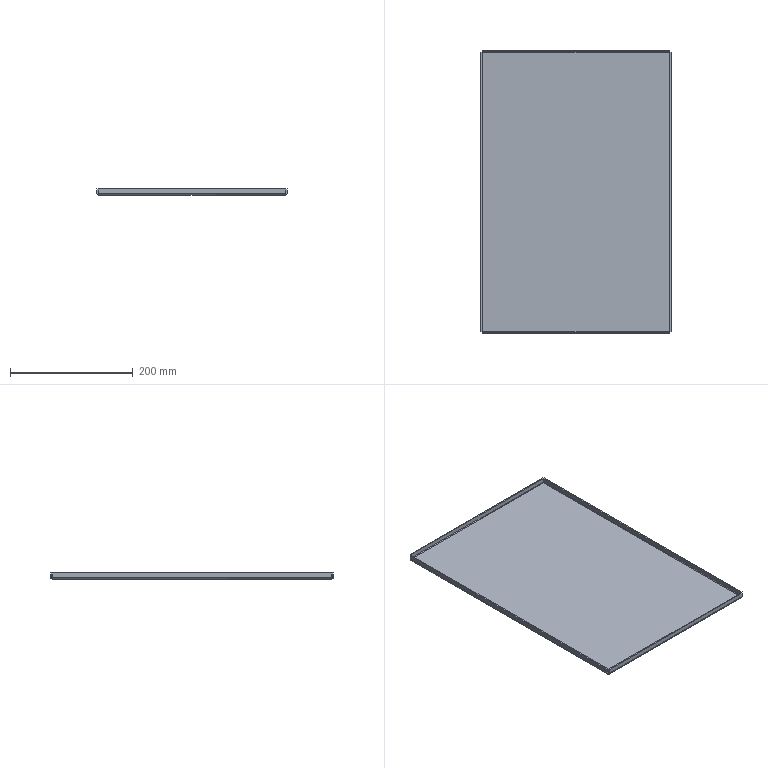Part | SolidWorks | features EdgeFlange 1, FlatPattern 1, SMBaseFlange 1, SheetMetal 1 | 1 solid | 38 faces | box 310 x 460 x 10 mm | volume 306822 mm3 | plane 22 | spline 8 | cylinder 8 | commonest cylinder face diameters 2 x4 6 x4
STEP:
#1=CARTESIAN_POINT('',(152.,-227.,-2.));
#2=VERTEX_POINT('',#1);
#3=CARTESIAN_POINT('',(-152.,-227.,-2.));
#4=VERTEX_POINT('',#3);
#5=CARTESIAN_POINT('',(152.293,-227.,-2.));
#6=DIRECTION('',(-1.,0.,0.));
#7=VECTOR('',#6,1000.);
#8=LINE('',#5,#7);
#9=EDGE_CURVE('',#2,#4,#8,.T.);
#10=ORIENTED_EDGE('',*,*,#9,.T.);
#11=CARTESIAN_POINT('',(-152.,227.,-2.));
#12=VERTEX_POINT('',#11);
#13=CARTESIAN_POINT('',(-152.,-227.293,-2.));
#14=DIRECTION('',(0.,1.,0.));
#15=VECTOR('',#14,1000.);
#16=LINE('',#13,#15);
#17=EDGE_CURVE('',#4,#12,#16,.T.);
#18=ORIENTED_EDGE('',*,*,#17,.T.);
#19=CARTESIAN_POINT('',(152.,227.,-2.));
#20=VERTEX_POINT('',#19);
#21=CARTESIAN_POINT('',(-152.293,227.,-2.));
#22=DIRECTION('',(1.,0.,0.));
#23=VECTOR('',#22,1000.);
#24=LINE('',#21,#23);
#25=EDGE_CURVE('',#12,#20,#24,.T.);
#26=ORIENTED_EDGE('',*,*,#25,.T.);
#27=CARTESIAN_POINT('',(152.,227.293,-2.));
#28=DIRECTION('',(0.,-1.,0.));
#29=VECTOR('',#28,1000.);
#30=LINE('',#27,#29);
#31=EDGE_CURVE('',#20,#2,#30,.T.);
#32=ORIENTED_EDGE('',*,*,#31,.T.);
#33=EDGE_LOOP('',(#10,#18,#26,#32));
#34=FACE_OUTER_BOUND('',#33,.T.);
#35=CARTESIAN_POINT('',(0.,0.,-2.));
#36=DIRECTION('',(0.,0.,1.));
#37=DIRECTION('',(1.,0.,0.));
#38=AXIS2_PLACEMENT_3D('',#35,#36,#37);
#39=PLANE('',#38);
#40=ADVANCED_FACE('',(#34),#39,.F.);
#41=CARTESIAN_POINT('',(-152.,-227.,0.));
#42=VERTEX_POINT('',#41);
#43=CARTESIAN_POINT('',(-152.,227.,0.));
#44=VERTEX_POINT('',#43);
#45=CARTESIAN_POINT('',(-152.,-227.293,0.));
#46=DIRECTION('',(0.,1.,0.));
#47=VECTOR('',#46,1000.);
#48=LINE('',#45,#47);
#49=EDGE_CURVE('',#42,#44,#48,.T.);
#50=ORIENTED_EDGE('',*,*,#49,.F.);
#51=CARTESIAN_POINT('',(152.,-227.,0.));
#52=VERTEX_POINT('',#51);
#53=CARTESIAN_POINT('',(152.293,-227.,0.));
#54=DIRECTION('',(-1.,0.,0.));
#55=VECTOR('',#54,1000.);
#56=LINE('',#53,#55);
#57=EDGE_CURVE('',#52,#42,#56,.T.);
#58=ORIENTED_EDGE('',*,*,#57,.F.);
#59=CARTESIAN_POINT('',(152.,227.,0.));
#60=VERTEX_POINT('',#59);
#61=CARTESIAN_POINT('',(152.,227.293,0.));
#62=DIRECTION('',(0.,-1.,0.));
#63=VECTOR('',#62,1000.);
#64=LINE('',#61,#63);
#65=EDGE_CURVE('',#60,#52,#64,.T.);
#66=ORIENTED_EDGE('',*,*,#65,.F.);
#67=CARTESIAN_POINT('',(-152.293,227.,0.));
#68=DIRECTION('',(1.,0.,0.));
#69=VECTOR('',#68,1000.);
#70=LINE('',#67,#69);
#71=EDGE_CURVE('',#44,#60,#70,.T.);
#72=ORIENTED_EDGE('',*,*,#71,.F.);
#73=EDGE_LOOP('',(#50,#58,#66,#72));
#74=FACE_OUTER_BOUND('',#73,.T.);
#75=CARTESIAN_POINT('',(0.,0.,0.));
#76=DIRECTION('',(0.,0.,1.));
#77=DIRECTION('',(1.,0.,0.));
#78=AXIS2_PLACEMENT_3D('',#75,#76,#77);
#79=PLANE('',#78);
#80=ADVANCED_FACE('',(#74),#79,.T.);
#81=CARTESIAN_POINT('',(-155.,227.293,1.));
#82=VERTEX_POINT('',#81);
#83=CARTESIAN_POINT('',(-153.,227.293,1.));
#84=VERTEX_POINT('',#83);
#85=CARTESIAN_POINT('',(-153.,227.293,1.));
#86=DIRECTION('',(1.,0.,0.));
#87=VECTOR('',#86,1000.);
#88=LINE('',#85,#87);
#89=EDGE_CURVE('',#82,#84,#88,.T.);
#90=ORIENTED_EDGE('',*,*,#89,.T.);
#91=CARTESIAN_POINT('',(-152.,227.,0.));
#92=CARTESIAN_POINT('',(-152.262,227.049,0.));
#93=CARTESIAN_POINT('',(-152.522,227.098,0.1078));
#94=CARTESIAN_POINT('',(-152.892,227.195,0.478));
#95=CARTESIAN_POINT('',(-153.,227.244,0.7382));
#96=CARTESIAN_POINT('',(-153.,227.293,1.));
#97=B_SPLINE_CURVE_WITH_KNOTS('',3,(#91,#92,#93,#94,#95,#96),.UNSPECIFIED.,.F.,.F.,(4,2,4),(0.,0.5,1.),.UNSPECIFIED.);
#98=EDGE_CURVE('',#44,#84,#97,.T.);
#99=ORIENTED_EDGE('',*,*,#98,.F.);
#100=CARTESIAN_POINT('',(-152.,227.,0.));
#101=DIRECTION('',(0.,0.,-1.));
#102=VECTOR('',#101,1000.);
#103=LINE('',#100,#102);
#104=EDGE_CURVE('',#44,#12,#103,.T.);
#105=ORIENTED_EDGE('',*,*,#104,.T.);
#106=CARTESIAN_POINT('',(-152.,227.,-2.));
#107=CARTESIAN_POINT('',(-152.393,227.024,-2.));
#108=CARTESIAN_POINT('',(-152.785,227.049,-1.922));
#109=CARTESIAN_POINT('',(-153.511,227.098,-1.621));
#110=CARTESIAN_POINT('',(-153.844,227.122,-1.399));
#111=CARTESIAN_POINT('',(-154.399,227.171,-0.8436));
#112=CARTESIAN_POINT('',(-154.621,227.195,-0.5109));
#113=CARTESIAN_POINT('',(-154.922,227.244,0.2148));
#114=CARTESIAN_POINT('',(-155.,227.268,0.6073));
#115=CARTESIAN_POINT('',(-155.,227.293,1.));
#116=B_SPLINE_CURVE_WITH_KNOTS('',3,(#106,#107,#108,#109,#110,#111,#112,#113,#114,#115),.UNSPECIFIED.,.F.,.F.,(4,2,2,2,4),(0.,0.25,0.5,0.75,1.),.UNSPECIFIED.);
#117=EDGE_CURVE('',#12,#82,#116,.T.);
#118=ORIENTED_EDGE('',*,*,#117,.T.);
#119=EDGE_LOOP('',(#90,#99,#105,#118));
#120=FACE_OUTER_BOUND('',#119,.T.);
#121=CARTESIAN_POINT('',(-152.,227.,-2.02));
#122=CARTESIAN_POINT('',(-152.395,227.024,-2.02));
#123=CARTESIAN_POINT('',(-152.79,227.049,-1.941));
#124=CARTESIAN_POINT('',(-153.521,227.098,-1.639));
#125=CARTESIAN_POINT('',(-153.856,227.122,-1.415));
#126=CARTESIAN_POINT('',(-154.415,227.171,-0.8559));
#127=CARTESIAN_POINT('',(-154.639,227.195,-0.5209));
#128=CARTESIAN_POINT('',(-154.941,227.244,0.2095));
#129=CARTESIAN_POINT('',(-155.02,227.268,0.6046));
#130=CARTESIAN_POINT('',(-155.02,227.293,1.));
#131=CARTESIAN_POINT('',(-152.,227.,-2.));
#132=CARTESIAN_POINT('',(-152.393,227.024,-2.));
#133=CARTESIAN_POINT('',(-152.785,227.049,-1.922));
#134=CARTESIAN_POINT('',(-153.511,227.098,-1.621));
#135=CARTESIAN_POINT('',(-153.844,227.122,-1.399));
#136=CARTESIAN_POINT('',(-154.399,227.171,-0.8436));
#137=CARTESIAN_POINT('',(-154.621,227.195,-0.5109));
#138=CARTESIAN_POINT('',(-154.922,227.244,0.2148));
#139=CARTESIAN_POINT('',(-155.,227.268,0.6072));
#140=CARTESIAN_POINT('',(-155.,227.293,1.));
#141=CARTESIAN_POINT('',(-152.,227.,0.));
#142=CARTESIAN_POINT('',(-152.131,227.024,0.));
#143=CARTESIAN_POINT('',(-152.262,227.049,0.02603));
#144=CARTESIAN_POINT('',(-152.504,227.098,0.1262));
#145=CARTESIAN_POINT('',(-152.615,227.122,0.2003));
#146=CARTESIAN_POINT('',(-152.8,227.171,0.3855));
#147=CARTESIAN_POINT('',(-152.874,227.195,0.4964));
#148=CARTESIAN_POINT('',(-152.974,227.244,0.7383));
#149=CARTESIAN_POINT('',(-153.,227.268,0.8691));
#150=CARTESIAN_POINT('',(-153.,227.293,1.));
#151=CARTESIAN_POINT('',(-152.,227.,0.0202));
#152=CARTESIAN_POINT('',(-152.128,227.024,0.0202));
#153=CARTESIAN_POINT('',(-152.256,227.049,0.0457));
#154=CARTESIAN_POINT('',(-152.493,227.098,0.1439));
#155=CARTESIAN_POINT('',(-152.602,227.122,0.2165));
#156=CARTESIAN_POINT('',(-152.784,227.171,0.3979));
#157=CARTESIAN_POINT('',(-152.856,227.195,0.5066));
#158=CARTESIAN_POINT('',(-152.954,227.244,0.7435));
#159=CARTESIAN_POINT('',(-152.98,227.268,0.8717));
#160=CARTESIAN_POINT('',(-152.98,227.293,1.));
#161=B_SPLINE_SURFACE_WITH_KNOTS('',1,3,((#121,#122,#123,#124,#125,#126,#127,#128,#129,#130),(#131,#132,#133,#134,#135,#136,#137,#138,#139,#140),(#141,#142,#143,#144,#145,#146,#147,#148,#149,#150),(#151,#152,#153,#154,#155,#156,#157,#158,#159,#160)),.UNSPECIFIED.,.F.,.F.,.F.,(2,1,1,2),(4,2,2,2,4),(-0.01,0.,1.,1.01),(0.,0.25,0.5,0.75,1.),.UNSPECIFIED.);
#162=ADVANCED_FACE('',(#120),#161,.F.);
#163=CARTESIAN_POINT('',(-153.,-227.293,1.));
#164=VERTEX_POINT('',#163);
#165=CARTESIAN_POINT('',(-153.,-227.293,1.));
#166=CARTESIAN_POINT('',(-153.,-227.244,0.7382));
#167=CARTESIAN_POINT('',(-152.892,-227.195,0.478));
#168=CARTESIAN_POINT('',(-152.522,-227.098,0.1078));
#169=CARTESIAN_POINT('',(-152.262,-227.049,0.));
#170=CARTESIAN_POINT('',(-152.,-227.,0.));
#171=B_SPLINE_CURVE_WITH_KNOTS('',3,(#165,#166,#167,#168,#169,#170),.UNSPECIFIED.,.F.,.F.,(4,2,4),(0.,0.5,1.),.UNSPECIFIED.);
#172=EDGE_CURVE('',#164,#42,#171,.T.);
#173=ORIENTED_EDGE('',*,*,#172,.F.);
#174=CARTESIAN_POINT('',(-155.,-227.293,1.));
#175=VERTEX_POINT('',#174);
#176=CARTESIAN_POINT('',(-153.,-227.293,1.));
#177=DIRECTION('',(1.,0.,0.));
#178=VECTOR('',#177,1000.);
#179=LINE('',#176,#178);
#180=EDGE_CURVE('',#175,#164,#179,.T.);
#181=ORIENTED_EDGE('',*,*,#180,.F.);
#182=CARTESIAN_POINT('',(-155.,-227.293,1.));
#183=CARTESIAN_POINT('',(-155.,-227.268,0.6073));
#184=CARTESIAN_POINT('',(-154.922,-227.244,0.2148));
#185=CARTESIAN_POINT('',(-154.621,-227.195,-0.5109));
#186=CARTESIAN_POINT('',(-154.399,-227.171,-0.8436));
#187=CARTESIAN_POINT('',(-153.844,-227.122,-1.399));
#188=CARTESIAN_POINT('',(-153.511,-227.098,-1.621));
#189=CARTESIAN_POINT('',(-152.785,-227.049,-1.922));
#190=CARTESIAN_POINT('',(-152.393,-227.024,-2.));
#191=CARTESIAN_POINT('',(-152.,-227.,-2.));
#192=B_SPLINE_CURVE_WITH_KNOTS('',3,(#182,#183,#184,#185,#186,#187,#188,#189,#190,#191),.UNSPECIFIED.,.F.,.F.,(4,2,2,2,4),(0.,0.25,0.5,0.75,1.),.UNSPECIFIED.);
#193=EDGE_CURVE('',#175,#4,#192,.T.);
#194=ORIENTED_EDGE('',*,*,#193,.T.);
#195=CARTESIAN_POINT('',(-152.,-227.,0.));
#196=DIRECTION('',(0.,0.,-1.));
#197=VECTOR('',#196,1000.);
#198=LINE('',#195,#197);
#199=EDGE_CURVE('',#42,#4,#198,.T.);
#200=ORIENTED_EDGE('',*,*,#199,.F.);
#201=EDGE_LOOP('',(#173,#181,#194,#200));
#202=FACE_OUTER_BOUND('',#201,.T.);
#203=CARTESIAN_POINT('',(-155.02,-227.293,1.));
#204=CARTESIAN_POINT('',(-155.02,-227.268,0.6046));
#205=CARTESIAN_POINT('',(-154.941,-227.244,0.2095));
#206=CARTESIAN_POINT('',(-154.639,-227.195,-0.5209));
#207=CARTESIAN_POINT('',(-154.415,-227.171,-0.8559));
#208=CARTESIAN_POINT('',(-153.856,-227.122,-1.415));
#209=CARTESIAN_POINT('',(-153.521,-227.098,-1.639));
#210=CARTESIAN_POINT('',(-152.79,-227.049,-1.941));
#211=CARTESIAN_POINT('',(-152.395,-227.024,-2.02));
#212=CARTESIAN_POINT('',(-152.,-227.,-2.02));
#213=CARTESIAN_POINT('',(-155.,-227.293,1.));
#214=CARTESIAN_POINT('',(-155.,-227.268,0.6072));
#215=CARTESIAN_POINT('',(-154.922,-227.244,0.2148));
#216=CARTESIAN_POINT('',(-154.621,-227.195,-0.5109));
#217=CARTESIAN_POINT('',(-154.399,-227.171,-0.8436));
#218=CARTESIAN_POINT('',(-153.844,-227.122,-1.399));
#219=CARTESIAN_POINT('',(-153.511,-227.098,-1.621));
#220=CARTESIAN_POINT('',(-152.785,-227.049,-1.922));
#221=CARTESIAN_POINT('',(-152.393,-227.024,-2.));
#222=CARTESIAN_POINT('',(-152.,-227.,-2.));
#223=CARTESIAN_POINT('',(-153.,-227.293,1.));
#224=CARTESIAN_POINT('',(-153.,-227.268,0.8691));
#225=CARTESIAN_POINT('',(-152.974,-227.244,0.7383));
#226=CARTESIAN_POINT('',(-152.874,-227.195,0.4964));
#227=CARTESIAN_POINT('',(-152.8,-227.171,0.3855));
#228=CARTESIAN_POINT('',(-152.615,-227.122,0.2003));
#229=CARTESIAN_POINT('',(-152.504,-227.098,0.1262));
#230=CARTESIAN_POINT('',(-152.262,-227.049,0.02603));
#231=CARTESIAN_POINT('',(-152.131,-227.024,0.));
#232=CARTESIAN_POINT('',(-152.,-227.,0.));
#233=CARTESIAN_POINT('',(-152.98,-227.293,1.));
#234=CARTESIAN_POINT('',(-152.98,-227.268,0.8717));
#235=CARTESIAN_POINT('',(-152.954,-227.244,0.7435));
#236=CARTESIAN_POINT('',(-152.856,-227.195,0.5066));
#237=CARTESIAN_POINT('',(-152.784,-227.171,0.3979));
#238=CARTESIAN_POINT('',(-152.602,-227.122,0.2165));
#239=CARTESIAN_POINT('',(-152.493,-227.098,0.1439));
#240=CARTESIAN_POINT('',(-152.256,-227.049,0.0457));
#241=CARTESIAN_POINT('',(-152.128,-227.024,0.0202));
#242=CARTESIAN_POINT('',(-152.,-227.,0.0202));
#243=B_SPLINE_SURFACE_WITH_KNOTS('',1,3,((#203,#204,#205,#206,#207,#208,#209,#210,#211,#212),(#213,#214,#215,#216,#217,#218,#219,#220,#221,#222),(#223,#224,#225,#226,#227,#228,#229,#230,#231,#232),(#233,#234,#235,#236,#237,#238,#239,#240,#241,#242)),.UNSPECIFIED.,.F.,.F.,.F.,(2,1,1,2),(4,2,2,2,4),(-0.01,0.,1.,1.01),(0.,0.25,0.5,0.75,1.),.UNSPECIFIED.);
#244=ADVANCED_FACE('',(#202),#243,.F.);
#245=ORIENTED_EDGE('',*,*,#17,.F.);
#246=ORIENTED_EDGE('',*,*,#193,.F.);
#247=CARTESIAN_POINT('',(-155.,230.,1.));
#248=DIRECTION('',(0.,1.,0.));
#249=VECTOR('',#248,1000.);
#250=LINE('',#247,#249);
#251=EDGE_CURVE('',#175,#82,#250,.T.);
#252=ORIENTED_EDGE('',*,*,#251,.T.);
#253=ORIENTED_EDGE('',*,*,#117,.F.);
#254=EDGE_LOOP('',(#245,#246,#252,#253));
#255=FACE_OUTER_BOUND('',#254,.T.);
#256=CARTESIAN_POINT('',(-152.,-227.293,1.));
#257=DIRECTION('',(0.,-1.,0.));
#258=DIRECTION('',(-1.,0.,0.));
#259=AXIS2_PLACEMENT_3D('',#256,#257,#258);
#260=CYLINDRICAL_SURFACE('',#259,3.);
#261=ADVANCED_FACE('',(#255),#260,.T.);
#262=ORIENTED_EDGE('',*,*,#49,.T.);
#263=ORIENTED_EDGE('',*,*,#98,.T.);
#264=CARTESIAN_POINT('',(-153.,230.,1.));
#265=DIRECTION('',(0.,-1.,0.));
#266=VECTOR('',#265,1000.);
#267=LINE('',#264,#266);
#268=EDGE_CURVE('',#84,#164,#267,.T.);
#269=ORIENTED_EDGE('',*,*,#268,.T.);
#270=ORIENTED_EDGE('',*,*,#172,.T.);
#271=EDGE_LOOP('',(#262,#263,#269,#270));
#272=FACE_OUTER_BOUND('',#271,.T.);
#273=CARTESIAN_POINT('',(-152.,-227.293,1.));
#274=DIRECTION('',(0.,-1.,0.));
#275=DIRECTION('',(-1.,0.,0.));
#276=AXIS2_PLACEMENT_3D('',#273,#274,#275);
#277=CYLINDRICAL_SURFACE('',#276,1.);
#278=ADVANCED_FACE('',(#272),#277,.F.);
#279=CARTESIAN_POINT('',(-155.,227.293,8.));
#280=VERTEX_POINT('',#279);
#281=CARTESIAN_POINT('',(-155.,227.293,0.));
#282=DIRECTION('',(0.,0.,1.));
#283=VECTOR('',#282,1000.);
#284=LINE('',#281,#283);
#285=EDGE_CURVE('',#82,#280,#284,.T.);
#286=ORIENTED_EDGE('',*,*,#285,.T.);
#287=CARTESIAN_POINT('',(-153.,227.293,8.));
#288=VERTEX_POINT('',#287);
#289=CARTESIAN_POINT('',(-153.,227.293,8.));
#290=DIRECTION('',(1.,0.,0.));
#291=VECTOR('',#290,1000.);
#292=LINE('',#289,#291);
#293=EDGE_CURVE('',#280,#288,#292,.T.);
#294=ORIENTED_EDGE('',*,*,#293,.T.);
#295=CARTESIAN_POINT('',(-153.,227.293,0.));
#296=DIRECTION('',(0.,0.,1.));
#297=VECTOR('',#296,1000.);
#298=LINE('',#295,#297);
#299=EDGE_CURVE('',#84,#288,#298,.T.);
#300=ORIENTED_EDGE('',*,*,#299,.F.);
#301=ORIENTED_EDGE('',*,*,#89,.F.);
#302=EDGE_LOOP('',(#286,#294,#300,#301));
#303=FACE_OUTER_BOUND('',#302,.T.);
#304=CARTESIAN_POINT('',(-153.,227.293,0.));
#305=DIRECTION('',(0.,1.,0.));
#306=DIRECTION('',(0.,0.,1.));
#307=AXIS2_PLACEMENT_3D('',#304,#305,#306);
#308=PLANE('',#307);
#309=ADVANCED_FACE('',(#303),#308,.T.);
#310=ORIENTED_EDGE('',*,*,#251,.F.);
#311=CARTESIAN_POINT('',(-155.,-227.293,8.));
#312=VERTEX_POINT('',#311);
#313=CARTESIAN_POINT('',(-155.,-227.293,0.));
#314=DIRECTION('',(0.,0.,1.));
#315=VECTOR('',#314,1000.);
#316=LINE('',#313,#315);
#317=EDGE_CURVE('',#175,#312,#316,.T.);
#318=ORIENTED_EDGE('',*,*,#317,.T.);
#319=CARTESIAN_POINT('',(-155.,0.,8.));
#320=DIRECTION('',(0.,1.,0.));
#321=VECTOR('',#320,1000.);
#322=LINE('',#319,#321);
#323=EDGE_CURVE('',#312,#280,#322,.T.);
#324=ORIENTED_EDGE('',*,*,#323,.T.);
#325=ORIENTED_EDGE('',*,*,#285,.F.);
#326=EDGE_LOOP('',(#310,#318,#324,#325));
#327=FACE_OUTER_BOUND('',#326,.T.);
#328=CARTESIAN_POINT('',(-155.,0.,0.));
#329=DIRECTION('',(1.,0.,0.));
#330=DIRECTION('',(0.,0.,-1.));
#331=AXIS2_PLACEMENT_3D('',#328,#329,#330);
#332=PLANE('',#331);
#333=ADVANCED_FACE('',(#327),#332,.F.);
#334=CARTESIAN_POINT('',(-153.,-227.293,8.));
#335=VERTEX_POINT('',#334);
#336=CARTESIAN_POINT('',(-153.,-227.293,0.));
#337=DIRECTION('',(0.,0.,1.));
#338=VECTOR('',#337,1000.);
#339=LINE('',#336,#338);
#340=EDGE_CURVE('',#164,#335,#339,.T.);
#341=ORIENTED_EDGE('',*,*,#340,.F.);
#342=ORIENTED_EDGE('',*,*,#268,.F.);
#343=ORIENTED_EDGE('',*,*,#299,.T.);
#344=CARTESIAN_POINT('',(-153.,230.,8.));
#345=DIRECTION('',(0.,1.,0.));
#346=VECTOR('',#345,1000.);
#347=LINE('',#344,#346);
#348=EDGE_CURVE('',#335,#288,#347,.T.);
#349=ORIENTED_EDGE('',*,*,#348,.F.);
#350=EDGE_LOOP('',(#341,#342,#343,#349));
#351=FACE_OUTER_BOUND('',#350,.T.);
#352=CARTESIAN_POINT('',(-153.,0.,0.));
#353=DIRECTION('',(1.,0.,0.));
#354=DIRECTION('',(0.,0.,-1.));
#355=AXIS2_PLACEMENT_3D('',#352,#353,#354);
#356=PLANE('',#355);
#357=ADVANCED_FACE('',(#351),#356,.T.);
#358=ORIENTED_EDGE('',*,*,#323,.F.);
#359=CARTESIAN_POINT('',(-155.,-227.293,8.));
#360=DIRECTION('',(1.,0.,0.));
#361=VECTOR('',#360,1000.);
#362=LINE('',#359,#361);
#363=EDGE_CURVE('',#312,#335,#362,.T.);
#364=ORIENTED_EDGE('',*,*,#363,.T.);
#365=ORIENTED_EDGE('',*,*,#348,.T.);
#366=ORIENTED_EDGE('',*,*,#293,.F.);
#367=EDGE_LOOP('',(#358,#364,#365,#366));
#368=FACE_OUTER_BOUND('',#367,.T.);
#369=CARTESIAN_POINT('',(-155.,230.,8.));
#370=DIRECTION('',(0.,0.,-1.));
#371=DIRECTION('',(-1.,0.,0.));
#372=AXIS2_PLACEMENT_3D('',#369,#370,#371);
#373=PLANE('',#372);
#374=ADVANCED_FACE('',(#368),#373,.F.);
#375=ORIENTED_EDGE('',*,*,#363,.F.);
#376=ORIENTED_EDGE('',*,*,#317,.F.);
#377=ORIENTED_EDGE('',*,*,#180,.T.);
#378=ORIENTED_EDGE('',*,*,#340,.T.);
#379=EDGE_LOOP('',(#375,#376,#377,#378));
#380=FACE_OUTER_BOUND('',#379,.T.);
#381=CARTESIAN_POINT('',(-153.,-227.293,0.));
#382=DIRECTION('',(0.,1.,0.));
#383=DIRECTION('',(0.,0.,1.));
#384=AXIS2_PLACEMENT_3D('',#381,#382,#383);
#385=PLANE('',#384);
#386=ADVANCED_FACE('',(#380),#385,.F.);
#387=CARTESIAN_POINT('',(152.293,230.,1.));
#388=VERTEX_POINT('',#387);
#389=CARTESIAN_POINT('',(152.293,228.,1.));
#390=VERTEX_POINT('',#389);
#391=CARTESIAN_POINT('',(152.293,228.,1.));
#392=DIRECTION('',(0.,-1.,0.));
#393=VECTOR('',#392,1000.);
#394=LINE('',#391,#393);
#395=EDGE_CURVE('',#388,#390,#394,.T.);
#396=ORIENTED_EDGE('',*,*,#395,.T.);
#397=CARTESIAN_POINT('',(152.,227.,0.));
#398=CARTESIAN_POINT('',(152.049,227.262,0.));
#399=CARTESIAN_POINT('',(152.098,227.522,0.1078));
#400=CARTESIAN_POINT('',(152.195,227.892,0.478));
#401=CARTESIAN_POINT('',(152.244,228.,0.7382));
#402=CARTESIAN_POINT('',(152.293,228.,1.));
#403=B_SPLINE_CURVE_WITH_KNOTS('',3,(#397,#398,#399,#400,#401,#402),.UNSPECIFIED.,.F.,.F.,(4,2,4),(0.,0.5,1.),.UNSPECIFIED.);
#404=EDGE_CURVE('',#60,#390,#403,.T.);
#405=ORIENTED_EDGE('',*,*,#404,.F.);
#406=CARTESIAN_POINT('',(152.,227.,0.));
#407=DIRECTION('',(0.,0.,-1.));
#408=VECTOR('',#407,1000.);
#409=LINE('',#406,#408);
#410=EDGE_CURVE('',#60,#20,#409,.T.);
#411=ORIENTED_EDGE('',*,*,#410,.T.);
#412=CARTESIAN_POINT('',(152.,227.,-2.));
#413=CARTESIAN_POINT('',(152.024,227.393,-2.));
#414=CARTESIAN_POINT('',(152.049,227.785,-1.922));
#415=CARTESIAN_POINT('',(152.098,228.511,-1.621));
#416=CARTESIAN_POINT('',(152.122,228.844,-1.399));
#417=CARTESIAN_POINT('',(152.171,229.399,-0.8436));
#418=CARTESIAN_POINT('',(152.195,229.621,-0.5109));
#419=CARTESIAN_POINT('',(152.244,229.922,0.2148));
#420=CARTESIAN_POINT('',(152.268,230.,0.6073));
#421=CARTESIAN_POINT('',(152.293,230.,1.));
#422=B_SPLINE_CURVE_WITH_KNOTS('',3,(#412,#413,#414,#415,#416,#417,#418,#419,#420,#421),.UNSPECIFIED.,.F.,.F.,(4,2,2,2,4),(0.,0.25,0.5,0.75,1.),.UNSPECIFIED.);
#423=EDGE_CURVE('',#20,#388,#422,.T.);
#424=ORIENTED_EDGE('',*,*,#423,.T.);
#425=EDGE_LOOP('',(#396,#405,#411,#424));
#426=FACE_OUTER_BOUND('',#425,.T.);
#427=CARTESIAN_POINT('',(152.,227.,-2.02));
#428=CARTESIAN_POINT('',(152.024,227.395,-2.02));
#429=CARTESIAN_POINT('',(152.049,227.79,-1.941));
#430=CARTESIAN_POINT('',(152.098,228.521,-1.639));
#431=CARTESIAN_POINT('',(152.122,228.856,-1.415));
#432=CARTESIAN_POINT('',(152.171,229.415,-0.8559));
#433=CARTESIAN_POINT('',(152.195,229.639,-0.5209));
#434=CARTESIAN_POINT('',(152.244,229.941,0.2095));
#435=CARTESIAN_POINT('',(152.268,230.02,0.6046));
#436=CARTESIAN_POINT('',(152.293,230.02,1.));
#437=CARTESIAN_POINT('',(152.,227.,-2.));
#438=CARTESIAN_POINT('',(152.024,227.393,-2.));
#439=CARTESIAN_POINT('',(152.049,227.785,-1.922));
#440=CARTESIAN_POINT('',(152.098,228.511,-1.621));
#441=CARTESIAN_POINT('',(152.122,228.844,-1.399));
#442=CARTESIAN_POINT('',(152.171,229.399,-0.8436));
#443=CARTESIAN_POINT('',(152.195,229.621,-0.5109));
#444=CARTESIAN_POINT('',(152.244,229.922,0.2148));
#445=CARTESIAN_POINT('',(152.268,230.,0.6072));
#446=CARTESIAN_POINT('',(152.293,230.,1.));
#447=CARTESIAN_POINT('',(152.,227.,0.));
#448=CARTESIAN_POINT('',(152.024,227.131,0.));
#449=CARTESIAN_POINT('',(152.049,227.262,0.02603));
#450=CARTESIAN_POINT('',(152.098,227.504,0.1262));
#451=CARTESIAN_POINT('',(152.122,227.615,0.2003));
#452=CARTESIAN_POINT('',(152.171,227.8,0.3855));
#453=CARTESIAN_POINT('',(152.195,227.874,0.4964));
#454=CARTESIAN_POINT('',(152.244,227.974,0.7383));
#455=CARTESIAN_POINT('',(152.268,228.,0.8691));
#456=CARTESIAN_POINT('',(152.293,228.,1.));
#457=CARTESIAN_POINT('',(152.,227.,0.0202));
#458=CARTESIAN_POINT('',(152.024,227.128,0.0202));
#459=CARTESIAN_POINT('',(152.049,227.256,0.0457));
#460=CARTESIAN_POINT('',(152.098,227.493,0.1439));
#461=CARTESIAN_POINT('',(152.122,227.602,0.2165));
#462=CARTESIAN_POINT('',(152.171,227.784,0.3979));
#463=CARTESIAN_POINT('',(152.195,227.856,0.5066));
#464=CARTESIAN_POINT('',(152.244,227.954,0.7435));
#465=CARTESIAN_POINT('',(152.268,227.98,0.8717));
#466=CARTESIAN_POINT('',(152.293,227.98,1.));
#467=B_SPLINE_SURFACE_WITH_KNOTS('',1,3,((#427,#428,#429,#430,#431,#432,#433,#434,#435,#436),(#437,#438,#439,#440,#441,#442,#443,#444,#445,#446),(#447,#448,#449,#450,#451,#452,#453,#454,#455,#456),(#457,#458,#459,#460,#461,#462,#463,#464,#465,#466)),.UNSPECIFIED.,.F.,.F.,.F.,(2,1,1,2),(4,2,2,2,4),(-0.01,0.,1.,1.01),(0.,0.25,0.5,0.75,1.),.UNSPECIFIED.);
#468=ADVANCED_FACE('',(#426),#467,.F.);
#469=CARTESIAN_POINT('',(-152.293,228.,1.));
#470=VERTEX_POINT('',#469);
#471=CARTESIAN_POINT('',(-152.293,228.,1.));
#472=CARTESIAN_POINT('',(-152.244,228.,0.7382));
#473=CARTESIAN_POINT('',(-152.195,227.892,0.478));
#474=CARTESIAN_POINT('',(-152.098,227.522,0.1078));
#475=CARTESIAN_POINT('',(-152.049,227.262,0.));
#476=CARTESIAN_POINT('',(-152.,227.,0.));
#477=B_SPLINE_CURVE_WITH_KNOTS('',3,(#471,#472,#473,#474,#475,#476),.UNSPECIFIED.,.F.,.F.,(4,2,4),(0.,0.5,1.),.UNSPECIFIED.);
#478=EDGE_CURVE('',#470,#44,#477,.T.);
#479=ORIENTED_EDGE('',*,*,#478,.F.);
#480=CARTESIAN_POINT('',(-152.293,230.,1.));
#481=VERTEX_POINT('',#480);
#482=CARTESIAN_POINT('',(-152.293,228.,1.));
#483=DIRECTION('',(0.,-1.,0.));
#484=VECTOR('',#483,1000.);
#485=LINE('',#482,#484);
#486=EDGE_CURVE('',#481,#470,#485,.T.);
#487=ORIENTED_EDGE('',*,*,#486,.F.);
#488=CARTESIAN_POINT('',(-152.293,230.,1.));
#489=CARTESIAN_POINT('',(-152.268,230.,0.6073));
#490=CARTESIAN_POINT('',(-152.244,229.922,0.2148));
#491=CARTESIAN_POINT('',(-152.195,229.621,-0.5109));
#492=CARTESIAN_POINT('',(-152.171,229.399,-0.8436));
#493=CARTESIAN_POINT('',(-152.122,228.844,-1.399));
#494=CARTESIAN_POINT('',(-152.098,228.511,-1.621));
#495=CARTESIAN_POINT('',(-152.049,227.785,-1.922));
#496=CARTESIAN_POINT('',(-152.024,227.393,-2.));
#497=CARTESIAN_POINT('',(-152.,227.,-2.));
#498=B_SPLINE_CURVE_WITH_KNOTS('',3,(#488,#489,#490,#491,#492,#493,#494,#495,#496,#497),.UNSPECIFIED.,.F.,.F.,(4,2,2,2,4),(0.,0.25,0.5,0.75,1.),.UNSPECIFIED.);
#499=EDGE_CURVE('',#481,#12,#498,.T.);
#500=ORIENTED_EDGE('',*,*,#499,.T.);
#501=ORIENTED_EDGE('',*,*,#104,.F.);
#502=EDGE_LOOP('',(#479,#487,#500,#501));
#503=FACE_OUTER_BOUND('',#502,.T.);
#504=CARTESIAN_POINT('',(-152.293,230.02,1.));
#505=CARTESIAN_POINT('',(-152.268,230.02,0.6046));
#506=CARTESIAN_POINT('',(-152.244,229.941,0.2095));
#507=CARTESIAN_POINT('',(-152.195,229.639,-0.5209));
#508=CARTESIAN_POINT('',(-152.171,229.415,-0.8559));
#509=CARTESIAN_POINT('',(-152.122,228.856,-1.415));
#510=CARTESIAN_POINT('',(-152.098,228.521,-1.639));
#511=CARTESIAN_POINT('',(-152.049,227.79,-1.941));
#512=CARTESIAN_POINT('',(-152.024,227.395,-2.02));
#513=CARTESIAN_POINT('',(-152.,227.,-2.02));
#514=CARTESIAN_POINT('',(-152.293,230.,1.));
#515=CARTESIAN_POINT('',(-152.268,230.,0.6072));
#516=CARTESIAN_POINT('',(-152.244,229.922,0.2148));
#517=CARTESIAN_POINT('',(-152.195,229.621,-0.5109));
#518=CARTESIAN_POINT('',(-152.171,229.399,-0.8436));
#519=CARTESIAN_POINT('',(-152.122,228.844,-1.399));
#520=CARTESIAN_POINT('',(-152.098,228.511,-1.621));
#521=CARTESIAN_POINT('',(-152.049,227.785,-1.922));
#522=CARTESIAN_POINT('',(-152.024,227.393,-2.));
#523=CARTESIAN_POINT('',(-152.,227.,-2.));
#524=CARTESIAN_POINT('',(-152.293,228.,1.));
#525=CARTESIAN_POINT('',(-152.268,228.,0.8691));
#526=CARTESIAN_POINT('',(-152.244,227.974,0.7383));
#527=CARTESIAN_POINT('',(-152.195,227.874,0.4964));
#528=CARTESIAN_POINT('',(-152.171,227.8,0.3855));
#529=CARTESIAN_POINT('',(-152.122,227.615,0.2003));
#530=CARTESIAN_POINT('',(-152.098,227.504,0.1262));
#531=CARTESIAN_POINT('',(-152.049,227.262,0.02603));
#532=CARTESIAN_POINT('',(-152.024,227.131,0.));
#533=CARTESIAN_POINT('',(-152.,227.,0.));
#534=CARTESIAN_POINT('',(-152.293,227.98,1.));
#535=CARTESIAN_POINT('',(-152.268,227.98,0.8717));
#536=CARTESIAN_POINT('',(-152.244,227.954,0.7435));
#537=CARTESIAN_POINT('',(-152.195,227.856,0.5066));
#538=CARTESIAN_POINT('',(-152.171,227.784,0.3979));
#539=CARTESIAN_POINT('',(-152.122,227.602,0.2165));
#540=CARTESIAN_POINT('',(-152.098,227.493,0.1439));
#541=CARTESIAN_POINT('',(-152.049,227.256,0.0457));
#542=CARTESIAN_POINT('',(-152.024,227.128,0.0202));
#543=CARTESIAN_POINT('',(-152.,227.,0.0202));
#544=B_SPLINE_SURFACE_WITH_KNOTS('',1,3,((#504,#505,#506,#507,#508,#509,#510,#511,#512,#513),(#514,#515,#516,#517,#518,#519,#520,#521,#522,#523),(#524,#525,#526,#527,#528,#529,#530,#531,#532,#533),(#534,#535,#536,#537,#538,#539,#540,#541,#542,#543)),.UNSPECIFIED.,.F.,.F.,.F.,(2,1,1,2),(4,2,2,2,4),(-0.01,0.,1.,1.01),(0.,0.25,0.5,0.75,1.),.UNSPECIFIED.);
#545=ADVANCED_FACE('',(#503),#544,.F.);
#546=ORIENTED_EDGE('',*,*,#25,.F.);
#547=ORIENTED_EDGE('',*,*,#499,.F.);
#548=CARTESIAN_POINT('',(155.,230.,1.));
#549=DIRECTION('',(1.,0.,0.));
#550=VECTOR('',#549,1000.);
#551=LINE('',#548,#550);
#552=EDGE_CURVE('',#481,#388,#551,.T.);
#553=ORIENTED_EDGE('',*,*,#552,.T.);
#554=ORIENTED_EDGE('',*,*,#423,.F.);
#555=EDGE_LOOP('',(#546,#547,#553,#554));
#556=FACE_OUTER_BOUND('',#555,.T.);
#557=CARTESIAN_POINT('',(-152.293,227.,1.));
#558=DIRECTION('',(-1.,0.,0.));
#559=DIRECTION('',(0.,1.,0.));
#560=AXIS2_PLACEMENT_3D('',#557,#558,#559);
#561=CYLINDRICAL_SURFACE('',#560,3.);
#562=ADVANCED_FACE('',(#556),#561,.T.);
#563=ORIENTED_EDGE('',*,*,#71,.T.);
#564=ORIENTED_EDGE('',*,*,#404,.T.);
#565=CARTESIAN_POINT('',(155.,228.,1.));
#566=DIRECTION('',(-1.,0.,0.));
#567=VECTOR('',#566,1000.);
#568=LINE('',#565,#567);
#569=EDGE_CURVE('',#390,#470,#568,.T.);
#570=ORIENTED_EDGE('',*,*,#569,.T.);
#571=ORIENTED_EDGE('',*,*,#478,.T.);
#572=EDGE_LOOP('',(#563,#564,#570,#571));
#573=FACE_OUTER_BOUND('',#572,.T.);
#574=CARTESIAN_POINT('',(-152.293,227.,1.));
#575=DIRECTION('',(-1.,0.,0.));
#576=DIRECTION('',(0.,1.,0.));
#577=AXIS2_PLACEMENT_3D('',#574,#575,#576);
#578=CYLINDRICAL_SURFACE('',#577,1.);
#579=ADVANCED_FACE('',(#573),#578,.F.);
#580=CARTESIAN_POINT('',(152.293,230.,8.));
#581=VERTEX_POINT('',#580);
#582=CARTESIAN_POINT('',(152.293,230.,0.));
#583=DIRECTION('',(0.,0.,1.));
#584=VECTOR('',#583,1000.);
#585=LINE('',#582,#584);
#586=EDGE_CURVE('',#388,#581,#585,.T.);
#587=ORIENTED_EDGE('',*,*,#586,.T.);
#588=CARTESIAN_POINT('',(152.293,228.,8.));
#589=VERTEX_POINT('',#588);
#590=CARTESIAN_POINT('',(152.293,228.,8.));
#591=DIRECTION('',(0.,-1.,0.));
#592=VECTOR('',#591,1000.);
#593=LINE('',#590,#592);
#594=EDGE_CURVE('',#581,#589,#593,.T.);
#595=ORIENTED_EDGE('',*,*,#594,.T.);
#596=CARTESIAN_POINT('',(152.293,228.,0.));
#597=DIRECTION('',(0.,0.,1.));
#598=VECTOR('',#597,1000.);
#599=LINE('',#596,#598);
#600=EDGE_CURVE('',#390,#589,#599,.T.);
#601=ORIENTED_EDGE('',*,*,#600,.F.);
#602=ORIENTED_EDGE('',*,*,#395,.F.);
#603=EDGE_LOOP('',(#587,#595,#601,#602));
#604=FACE_OUTER_BOUND('',#603,.T.);
#605=CARTESIAN_POINT('',(152.293,228.,0.));
#606=DIRECTION('',(1.,0.,0.));
#607=DIRECTION('',(0.,0.,-1.));
#608=AXIS2_PLACEMENT_3D('',#605,#606,#607);
#609=PLANE('',#608);
#610=ADVANCED_FACE('',(#604),#609,.T.);
#611=ORIENTED_EDGE('',*,*,#552,.F.);
#612=CARTESIAN_POINT('',(-152.293,230.,8.));
#613=VERTEX_POINT('',#612);
#614=CARTESIAN_POINT('',(-152.293,230.,0.));
#615=DIRECTION('',(0.,0.,1.));
#616=VECTOR('',#615,1000.);
#617=LINE('',#614,#616);
#618=EDGE_CURVE('',#481,#613,#617,.T.);
#619=ORIENTED_EDGE('',*,*,#618,.T.);
#620=CARTESIAN_POINT('',(0.,230.,8.));
#621=DIRECTION('',(1.,0.,0.));
#622=VECTOR('',#621,1000.);
#623=LINE('',#620,#622);
#624=EDGE_CURVE('',#613,#581,#623,.T.);
#625=ORIENTED_EDGE('',*,*,#624,.T.);
#626=ORIENTED_EDGE('',*,*,#586,.F.);
#627=EDGE_LOOP('',(#611,#619,#625,#626));
#628=FACE_OUTER_BOUND('',#627,.T.);
#629=CARTESIAN_POINT('',(0.,230.,0.));
#630=DIRECTION('',(0.,-1.,0.));
#631=DIRECTION('',(0.,0.,-1.));
#632=AXIS2_PLACEMENT_3D('',#629,#630,#631);
#633=PLANE('',#632);
#634=ADVANCED_FACE('',(#628),#633,.F.);
#635=CARTESIAN_POINT('',(-152.293,228.,8.));
#636=VERTEX_POINT('',#635);
#637=CARTESIAN_POINT('',(-152.293,228.,0.));
#638=DIRECTION('',(0.,0.,1.));
#639=VECTOR('',#638,1000.);
#640=LINE('',#637,#639);
#641=EDGE_CURVE('',#470,#636,#640,.T.);
#642=ORIENTED_EDGE('',*,*,#641,.F.);
#643=ORIENTED_EDGE('',*,*,#569,.F.);
#644=ORIENTED_EDGE('',*,*,#600,.T.);
#645=CARTESIAN_POINT('',(155.,228.,8.));
#646=DIRECTION('',(1.,0.,0.));
#647=VECTOR('',#646,1000.);
#648=LINE('',#645,#647);
#649=EDGE_CURVE('',#636,#589,#648,.T.);
#650=ORIENTED_EDGE('',*,*,#649,.F.);
#651=EDGE_LOOP('',(#642,#643,#644,#650));
#652=FACE_OUTER_BOUND('',#651,.T.);
#653=CARTESIAN_POINT('',(0.,228.,0.));
#654=DIRECTION('',(0.,-1.,0.));
#655=DIRECTION('',(0.,0.,-1.));
#656=AXIS2_PLACEMENT_3D('',#653,#654,#655);
#657=PLANE('',#656);
#658=ADVANCED_FACE('',(#652),#657,.T.);
#659=ORIENTED_EDGE('',*,*,#624,.F.);
#660=CARTESIAN_POINT('',(-152.293,230.,8.));
#661=DIRECTION('',(0.,-1.,0.));
#662=VECTOR('',#661,1000.);
#663=LINE('',#660,#662);
#664=EDGE_CURVE('',#613,#636,#663,.T.);
#665=ORIENTED_EDGE('',*,*,#664,.T.);
#666=ORIENTED_EDGE('',*,*,#649,.T.);
#667=ORIENTED_EDGE('',*,*,#594,.F.);
#668=EDGE_LOOP('',(#659,#665,#666,#667));
#669=FACE_OUTER_BOUND('',#668,.T.);
#670=CARTESIAN_POINT('',(155.,230.,8.));
#671=DIRECTION('',(0.,0.,-1.));
#672=DIRECTION('',(0.,1.,0.));
#673=AXIS2_PLACEMENT_3D('',#670,#671,#672);
#674=PLANE('',#673);
#675=ADVANCED_FACE('',(#669),#674,.F.);
#676=ORIENTED_EDGE('',*,*,#664,.F.);
#677=ORIENTED_EDGE('',*,*,#618,.F.);
#678=ORIENTED_EDGE('',*,*,#486,.T.);
#679=ORIENTED_EDGE('',*,*,#641,.T.);
#680=EDGE_LOOP('',(#676,#677,#678,#679));
#681=FACE_OUTER_BOUND('',#680,.T.);
#682=CARTESIAN_POINT('',(-152.293,228.,0.));
#683=DIRECTION('',(1.,0.,0.));
#684=DIRECTION('',(0.,0.,-1.));
#685=AXIS2_PLACEMENT_3D('',#682,#683,#684);
#686=PLANE('',#685);
#687=ADVANCED_FACE('',(#681),#686,.F.);
#688=CARTESIAN_POINT('',(155.,-227.293,1.));
#689=VERTEX_POINT('',#688);
#690=CARTESIAN_POINT('',(153.,-227.293,1.));
#691=VERTEX_POINT('',#690);
#692=CARTESIAN_POINT('',(153.,-227.293,1.));
#693=DIRECTION('',(-1.,0.,0.));
#694=VECTOR('',#693,1000.);
#695=LINE('',#692,#694);
#696=EDGE_CURVE('',#689,#691,#695,.T.);
#697=ORIENTED_EDGE('',*,*,#696,.T.);
#698=CARTESIAN_POINT('',(152.,-227.,0.));
#699=CARTESIAN_POINT('',(152.262,-227.049,0.));
#700=CARTESIAN_POINT('',(152.522,-227.098,0.1078));
#701=CARTESIAN_POINT('',(152.892,-227.195,0.478));
#702=CARTESIAN_POINT('',(153.,-227.244,0.7382));
#703=CARTESIAN_POINT('',(153.,-227.293,1.));
#704=B_SPLINE_CURVE_WITH_KNOTS('',3,(#698,#699,#700,#701,#702,#703),.UNSPECIFIED.,.F.,.F.,(4,2,4),(0.,0.5,1.),.UNSPECIFIED.);
#705=EDGE_CURVE('',#52,#691,#704,.T.);
#706=ORIENTED_EDGE('',*,*,#705,.F.);
#707=CARTESIAN_POINT('',(152.,-227.,0.));
#708=DIRECTION('',(0.,0.,-1.));
#709=VECTOR('',#708,1000.);
#710=LINE('',#707,#709);
#711=EDGE_CURVE('',#52,#2,#710,.T.);
#712=ORIENTED_EDGE('',*,*,#711,.T.);
#713=CARTESIAN_POINT('',(152.,-227.,-2.));
#714=CARTESIAN_POINT('',(152.393,-227.024,-2.));
#715=CARTESIAN_POINT('',(152.785,-227.049,-1.922));
#716=CARTESIAN_POINT('',(153.511,-227.098,-1.621));
#717=CARTESIAN_POINT('',(153.844,-227.122,-1.399));
#718=CARTESIAN_POINT('',(154.399,-227.171,-0.8436));
#719=CARTESIAN_POINT('',(154.621,-227.195,-0.5109));
#720=CARTESIAN_POINT('',(154.922,-227.244,0.2148));
#721=CARTESIAN_POINT('',(155.,-227.268,0.6073));
#722=CARTESIAN_POINT('',(155.,-227.293,1.));
#723=B_SPLINE_CURVE_WITH_KNOTS('',3,(#713,#714,#715,#716,#717,#718,#719,#720,#721,#722),.UNSPECIFIED.,.F.,.F.,(4,2,2,2,4),(0.,0.25,0.5,0.75,1.),.UNSPECIFIED.);
#724=EDGE_CURVE('',#2,#689,#723,.T.);
#725=ORIENTED_EDGE('',*,*,#724,.T.);
#726=EDGE_LOOP('',(#697,#706,#712,#725));
#727=FACE_OUTER_BOUND('',#726,.T.);
#728=CARTESIAN_POINT('',(152.,-227.,-2.02));
#729=CARTESIAN_POINT('',(152.395,-227.024,-2.02));
#730=CARTESIAN_POINT('',(152.79,-227.049,-1.941));
#731=CARTESIAN_POINT('',(153.521,-227.098,-1.639));
#732=CARTESIAN_POINT('',(153.856,-227.122,-1.415));
#733=CARTESIAN_POINT('',(154.415,-227.171,-0.8559));
#734=CARTESIAN_POINT('',(154.639,-227.195,-0.5209));
#735=CARTESIAN_POINT('',(154.941,-227.244,0.2095));
#736=CARTESIAN_POINT('',(155.02,-227.268,0.6046));
#737=CARTESIAN_POINT('',(155.02,-227.293,1.));
#738=CARTESIAN_POINT('',(152.,-227.,-2.));
#739=CARTESIAN_POINT('',(152.393,-227.024,-2.));
#740=CARTESIAN_POINT('',(152.785,-227.049,-1.922));
#741=CARTESIAN_POINT('',(153.511,-227.098,-1.621));
#742=CARTESIAN_POINT('',(153.844,-227.122,-1.399));
#743=CARTESIAN_POINT('',(154.399,-227.171,-0.8436));
#744=CARTESIAN_POINT('',(154.621,-227.195,-0.5109));
#745=CARTESIAN_POINT('',(154.922,-227.244,0.2148));
#746=CARTESIAN_POINT('',(155.,-227.268,0.6072));
#747=CARTESIAN_POINT('',(155.,-227.293,1.));
#748=CARTESIAN_POINT('',(152.,-227.,0.));
#749=CARTESIAN_POINT('',(152.131,-227.024,0.));
#750=CARTESIAN_POINT('',(152.262,-227.049,0.02603));
#751=CARTESIAN_POINT('',(152.504,-227.098,0.1262));
#752=CARTESIAN_POINT('',(152.615,-227.122,0.2003));
#753=CARTESIAN_POINT('',(152.8,-227.171,0.3855));
#754=CARTESIAN_POINT('',(152.874,-227.195,0.4964));
#755=CARTESIAN_POINT('',(152.974,-227.244,0.7383));
#756=CARTESIAN_POINT('',(153.,-227.268,0.8691));
#757=CARTESIAN_POINT('',(153.,-227.293,1.));
#758=CARTESIAN_POINT('',(152.,-227.,0.0202));
#759=CARTESIAN_POINT('',(152.128,-227.024,0.0202));
#760=CARTESIAN_POINT('',(152.256,-227.049,0.0457));
#761=CARTESIAN_POINT('',(152.493,-227.098,0.1439));
#762=CARTESIAN_POINT('',(152.602,-227.122,0.2165));
#763=CARTESIAN_POINT('',(152.784,-227.171,0.3979));
#764=CARTESIAN_POINT('',(152.856,-227.195,0.5066));
#765=CARTESIAN_POINT('',(152.954,-227.244,0.7435));
#766=CARTESIAN_POINT('',(152.98,-227.268,0.8717));
#767=CARTESIAN_POINT('',(152.98,-227.293,1.));
#768=B_SPLINE_SURFACE_WITH_KNOTS('',1,3,((#728,#729,#730,#731,#732,#733,#734,#735,#736,#737),(#738,#739,#740,#741,#742,#743,#744,#745,#746,#747),(#748,#749,#750,#751,#752,#753,#754,#755,#756,#757),(#758,#759,#760,#761,#762,#763,#764,#765,#766,#767)),.UNSPECIFIED.,.F.,.F.,.F.,(2,1,1,2),(4,2,2,2,4),(-0.01,0.,1.,1.01),(0.,0.25,0.5,0.75,1.),.UNSPECIFIED.);
#769=ADVANCED_FACE('',(#727),#768,.F.);
#770=CARTESIAN_POINT('',(153.,227.293,1.));
#771=VERTEX_POINT('',#770);
#772=CARTESIAN_POINT('',(153.,227.293,1.));
#773=CARTESIAN_POINT('',(153.,227.244,0.7382));
#774=CARTESIAN_POINT('',(152.892,227.195,0.478));
#775=CARTESIAN_POINT('',(152.522,227.098,0.1078));
#776=CARTESIAN_POINT('',(152.262,227.049,0.));
#777=CARTESIAN_POINT('',(152.,227.,0.));
#778=B_SPLINE_CURVE_WITH_KNOTS('',3,(#772,#773,#774,#775,#776,#777),.UNSPECIFIED.,.F.,.F.,(4,2,4),(0.,0.5,1.),.UNSPECIFIED.);
#779=EDGE_CURVE('',#771,#60,#778,.T.);
#780=ORIENTED_EDGE('',*,*,#779,.F.);
#781=CARTESIAN_POINT('',(155.,227.293,1.));
#782=VERTEX_POINT('',#781);
#783=CARTESIAN_POINT('',(153.,227.293,1.));
#784=DIRECTION('',(-1.,0.,0.));
#785=VECTOR('',#784,1000.);
#786=LINE('',#783,#785);
#787=EDGE_CURVE('',#782,#771,#786,.T.);
#788=ORIENTED_EDGE('',*,*,#787,.F.);
#789=CARTESIAN_POINT('',(155.,227.293,1.));
#790=CARTESIAN_POINT('',(155.,227.268,0.6073));
#791=CARTESIAN_POINT('',(154.922,227.244,0.2148));
#792=CARTESIAN_POINT('',(154.621,227.195,-0.5109));
#793=CARTESIAN_POINT('',(154.399,227.171,-0.8436));
#794=CARTESIAN_POINT('',(153.844,227.122,-1.399));
#795=CARTESIAN_POINT('',(153.511,227.098,-1.621));
#796=CARTESIAN_POINT('',(152.785,227.049,-1.922));
#797=CARTESIAN_POINT('',(152.393,227.024,-2.));
#798=CARTESIAN_POINT('',(152.,227.,-2.));
#799=B_SPLINE_CURVE_WITH_KNOTS('',3,(#789,#790,#791,#792,#793,#794,#795,#796,#797,#798),.UNSPECIFIED.,.F.,.F.,(4,2,2,2,4),(0.,0.25,0.5,0.75,1.),.UNSPECIFIED.);
#800=EDGE_CURVE('',#782,#20,#799,.T.);
#801=ORIENTED_EDGE('',*,*,#800,.T.);
#802=ORIENTED_EDGE('',*,*,#410,.F.);
#803=EDGE_LOOP('',(#780,#788,#801,#802));
#804=FACE_OUTER_BOUND('',#803,.T.);
#805=CARTESIAN_POINT('',(155.02,227.293,1.));
#806=CARTESIAN_POINT('',(155.02,227.268,0.6046));
#807=CARTESIAN_POINT('',(154.941,227.244,0.2095));
#808=CARTESIAN_POINT('',(154.639,227.195,-0.5209));
#809=CARTESIAN_POINT('',(154.415,227.171,-0.8559));
#810=CARTESIAN_POINT('',(153.856,227.122,-1.415));
#811=CARTESIAN_POINT('',(153.521,227.098,-1.639));
#812=CARTESIAN_POINT('',(152.79,227.049,-1.941));
#813=CARTESIAN_POINT('',(152.395,227.024,-2.02));
#814=CARTESIAN_POINT('',(152.,227.,-2.02));
#815=CARTESIAN_POINT('',(155.,227.293,1.));
#816=CARTESIAN_POINT('',(155.,227.268,0.6072));
#817=CARTESIAN_POINT('',(154.922,227.244,0.2148));
#818=CARTESIAN_POINT('',(154.621,227.195,-0.5109));
#819=CARTESIAN_POINT('',(154.399,227.171,-0.8436));
#820=CARTESIAN_POINT('',(153.844,227.122,-1.399));
#821=CARTESIAN_POINT('',(153.511,227.098,-1.621));
#822=CARTESIAN_POINT('',(152.785,227.049,-1.922));
#823=CARTESIAN_POINT('',(152.393,227.024,-2.));
#824=CARTESIAN_POINT('',(152.,227.,-2.));
#825=CARTESIAN_POINT('',(153.,227.293,1.));
#826=CARTESIAN_POINT('',(153.,227.268,0.8691));
#827=CARTESIAN_POINT('',(152.974,227.244,0.7383));
#828=CARTESIAN_POINT('',(152.874,227.195,0.4964));
#829=CARTESIAN_POINT('',(152.8,227.171,0.3855));
#830=CARTESIAN_POINT('',(152.615,227.122,0.2003));
#831=CARTESIAN_POINT('',(152.504,227.098,0.1262));
#832=CARTESIAN_POINT('',(152.262,227.049,0.02603));
#833=CARTESIAN_POINT('',(152.131,227.024,0.));
#834=CARTESIAN_POINT('',(152.,227.,0.));
#835=CARTESIAN_POINT('',(152.98,227.293,1.));
#836=CARTESIAN_POINT('',(152.98,227.268,0.8717));
#837=CARTESIAN_POINT('',(152.954,227.244,0.7435));
#838=CARTESIAN_POINT('',(152.856,227.195,0.5066));
#839=CARTESIAN_POINT('',(152.784,227.171,0.3979));
#840=CARTESIAN_POINT('',(152.602,227.122,0.2165));
#841=CARTESIAN_POINT('',(152.493,227.098,0.1439));
#842=CARTESIAN_POINT('',(152.256,227.049,0.0457));
#843=CARTESIAN_POINT('',(152.128,227.024,0.0202));
#844=CARTESIAN_POINT('',(152.,227.,0.0202));
#845=B_SPLINE_SURFACE_WITH_KNOTS('',1,3,((#805,#806,#807,#808,#809,#810,#811,#812,#813,#814),(#815,#816,#817,#818,#819,#820,#821,#822,#823,#824),(#825,#826,#827,#828,#829,#830,#831,#832,#833,#834),(#835,#836,#837,#838,#839,#840,#841,#842,#843,#844)),.UNSPECIFIED.,.F.,.F.,.F.,(2,1,1,2),(4,2,2,2,4),(-0.01,0.,1.,1.01),(0.,0.25,0.5,0.75,1.),.UNSPECIFIED.);
#846=ADVANCED_FACE('',(#804),#845,.F.);
#847=ORIENTED_EDGE('',*,*,#31,.F.);
#848=ORIENTED_EDGE('',*,*,#800,.F.);
#849=CARTESIAN_POINT('',(155.,-230.,1.));
#850=DIRECTION('',(0.,-1.,0.));
#851=VECTOR('',#850,1000.);
#852=LINE('',#849,#851);
#853=EDGE_CURVE('',#782,#689,#852,.T.);
#854=ORIENTED_EDGE('',*,*,#853,.T.);
#855=ORIENTED_EDGE('',*,*,#724,.F.);
#856=EDGE_LOOP('',(#847,#848,#854,#855));
#857=FACE_OUTER_BOUND('',#856,.T.);
#858=CARTESIAN_POINT('',(152.,227.293,1.));
#859=DIRECTION('',(0.,1.,0.));
#860=DIRECTION('',(1.,0.,0.));
#861=AXIS2_PLACEMENT_3D('',#858,#859,#860);
#862=CYLINDRICAL_SURFACE('',#861,3.);
#863=ADVANCED_FACE('',(#857),#862,.T.);
#864=ORIENTED_EDGE('',*,*,#65,.T.);
#865=ORIENTED_EDGE('',*,*,#705,.T.);
#866=CARTESIAN_POINT('',(153.,-230.,1.));
#867=DIRECTION('',(0.,1.,0.));
#868=VECTOR('',#867,1000.);
#869=LINE('',#866,#868);
#870=EDGE_CURVE('',#691,#771,#869,.T.);
#871=ORIENTED_EDGE('',*,*,#870,.T.);
#872=ORIENTED_EDGE('',*,*,#779,.T.);
#873=EDGE_LOOP('',(#864,#865,#871,#872));
#874=FACE_OUTER_BOUND('',#873,.T.);
#875=CARTESIAN_POINT('',(152.,227.293,1.));
#876=DIRECTION('',(0.,1.,0.));
#877=DIRECTION('',(1.,0.,0.));
#878=AXIS2_PLACEMENT_3D('',#875,#876,#877);
#879=CYLINDRICAL_SURFACE('',#878,1.);
#880=ADVANCED_FACE('',(#874),#879,.F.);
#881=CARTESIAN_POINT('',(155.,-227.293,8.));
#882=VERTEX_POINT('',#881);
#883=CARTESIAN_POINT('',(155.,-227.293,0.));
#884=DIRECTION('',(0.,0.,1.));
#885=VECTOR('',#884,1000.);
#886=LINE('',#883,#885);
#887=EDGE_CURVE('',#689,#882,#886,.T.);
#888=ORIENTED_EDGE('',*,*,#887,.T.);
#889=CARTESIAN_POINT('',(153.,-227.293,8.));
#890=VERTEX_POINT('',#889);
#891=CARTESIAN_POINT('',(153.,-227.293,8.));
#892=DIRECTION('',(-1.,0.,0.));
#893=VECTOR('',#892,1000.);
#894=LINE('',#891,#893);
#895=EDGE_CURVE('',#882,#890,#894,.T.);
#896=ORIENTED_EDGE('',*,*,#895,.T.);
#897=CARTESIAN_POINT('',(153.,-227.293,0.));
#898=DIRECTION('',(0.,0.,1.));
#899=VECTOR('',#898,1000.);
#900=LINE('',#897,#899);
#901=EDGE_CURVE('',#691,#890,#900,.T.);
#902=ORIENTED_EDGE('',*,*,#901,.F.);
#903=ORIENTED_EDGE('',*,*,#696,.F.);
#904=EDGE_LOOP('',(#888,#896,#902,#903));
#905=FACE_OUTER_BOUND('',#904,.T.);
#906=CARTESIAN_POINT('',(153.,-227.293,0.));
#907=DIRECTION('',(0.,-1.,0.));
#908=DIRECTION('',(0.,0.,-1.));
#909=AXIS2_PLACEMENT_3D('',#906,#907,#908);
#910=PLANE('',#909);
#911=ADVANCED_FACE('',(#905),#910,.T.);
#912=ORIENTED_EDGE('',*,*,#853,.F.);
#913=CARTESIAN_POINT('',(155.,227.293,8.));
#914=VERTEX_POINT('',#913);
#915=CARTESIAN_POINT('',(155.,227.293,0.));
#916=DIRECTION('',(0.,0.,1.));
#917=VECTOR('',#916,1000.);
#918=LINE('',#915,#917);
#919=EDGE_CURVE('',#782,#914,#918,.T.);
#920=ORIENTED_EDGE('',*,*,#919,.T.);
#921=CARTESIAN_POINT('',(155.,0.,8.));
#922=DIRECTION('',(0.,-1.,0.));
#923=VECTOR('',#922,1000.);
#924=LINE('',#921,#923);
#925=EDGE_CURVE('',#914,#882,#924,.T.);
#926=ORIENTED_EDGE('',*,*,#925,.T.);
#927=ORIENTED_EDGE('',*,*,#887,.F.);
#928=EDGE_LOOP('',(#912,#920,#926,#927));
#929=FACE_OUTER_BOUND('',#928,.T.);
#930=CARTESIAN_POINT('',(155.,0.,0.));
#931=DIRECTION('',(-1.,0.,0.));
#932=DIRECTION('',(0.,0.,1.));
#933=AXIS2_PLACEMENT_3D('',#930,#931,#932);
#934=PLANE('',#933);
#935=ADVANCED_FACE('',(#929),#934,.F.);
#936=CARTESIAN_POINT('',(153.,227.293,8.));
#937=VERTEX_POINT('',#936);
#938=CARTESIAN_POINT('',(153.,227.293,0.));
#939=DIRECTION('',(0.,0.,1.));
#940=VECTOR('',#939,1000.);
#941=LINE('',#938,#940);
#942=EDGE_CURVE('',#771,#937,#941,.T.);
#943=ORIENTED_EDGE('',*,*,#942,.F.);
#944=ORIENTED_EDGE('',*,*,#870,.F.);
#945=ORIENTED_EDGE('',*,*,#901,.T.);
#946=CARTESIAN_POINT('',(153.,-230.,8.));
#947=DIRECTION('',(0.,-1.,0.));
#948=VECTOR('',#947,1000.);
#949=LINE('',#946,#948);
#950=EDGE_CURVE('',#937,#890,#949,.T.);
#951=ORIENTED_EDGE('',*,*,#950,.F.);
#952=EDGE_LOOP('',(#943,#944,#945,#951));
#953=FACE_OUTER_BOUND('',#952,.T.);
#954=CARTESIAN_POINT('',(153.,0.,0.));
#955=DIRECTION('',(-1.,0.,0.));
#956=DIRECTION('',(0.,0.,1.));
#957=AXIS2_PLACEMENT_3D('',#954,#955,#956);
#958=PLANE('',#957);
#959=ADVANCED_FACE('',(#953),#958,.T.);
#960=ORIENTED_EDGE('',*,*,#925,.F.);
#961=CARTESIAN_POINT('',(155.,227.293,8.));
#962=DIRECTION('',(-1.,0.,0.));
#963=VECTOR('',#962,1000.);
#964=LINE('',#961,#963);
#965=EDGE_CURVE('',#914,#937,#964,.T.);
#966=ORIENTED_EDGE('',*,*,#965,.T.);
#967=ORIENTED_EDGE('',*,*,#950,.T.);
#968=ORIENTED_EDGE('',*,*,#895,.F.);
#969=EDGE_LOOP('',(#960,#966,#967,#968));
#970=FACE_OUTER_BOUND('',#969,.T.);
#971=CARTESIAN_POINT('',(155.,-230.,8.));
#972=DIRECTION('',(0.,0.,-1.));
#973=DIRECTION('',(-1.,0.,0.));
#974=AXIS2_PLACEMENT_3D('',#971,#972,#973);
#975=PLANE('',#974);
#976=ADVANCED_FACE('',(#970),#975,.F.);
#977=ORIENTED_EDGE('',*,*,#965,.F.);
#978=ORIENTED_EDGE('',*,*,#919,.F.);
#979=ORIENTED_EDGE('',*,*,#787,.T.);
#980=ORIENTED_EDGE('',*,*,#942,.T.);
#981=EDGE_LOOP('',(#977,#978,#979,#980));
#982=FACE_OUTER_BOUND('',#981,.T.);
#983=CARTESIAN_POINT('',(153.,227.293,0.));
#984=DIRECTION('',(0.,-1.,0.));
#985=DIRECTION('',(0.,0.,-1.));
#986=AXIS2_PLACEMENT_3D('',#983,#984,#985);
#987=PLANE('',#986);
#988=ADVANCED_FACE('',(#982),#987,.F.);
#989=CARTESIAN_POINT('',(-152.293,-230.,1.));
#990=VERTEX_POINT('',#989);
#991=CARTESIAN_POINT('',(-152.293,-228.,1.));
#992=VERTEX_POINT('',#991);
#993=CARTESIAN_POINT('',(-152.293,-228.,1.));
#994=DIRECTION('',(0.,1.,0.));
#995=VECTOR('',#994,1000.);
#996=LINE('',#993,#995);
#997=EDGE_CURVE('',#990,#992,#996,.T.);
#998=ORIENTED_EDGE('',*,*,#997,.T.);
#999=CARTESIAN_POINT('',(-152.,-227.,0.));
#1000=CARTESIAN_POINT('',(-152.049,-227.262,0.));
#1001=CARTESIAN_POINT('',(-152.098,-227.522,0.1078));
#1002=CARTESIAN_POINT('',(-152.195,-227.892,0.478));
#1003=CARTESIAN_POINT('',(-152.244,-228.,0.7382));
#1004=CARTESIAN_POINT('',(-152.293,-228.,1.));
#1005=B_SPLINE_CURVE_WITH_KNOTS('',3,(#999,#1000,#1001,#1002,#1003,#1004),.UNSPECIFIED.,.F.,.F.,(4,2,4),(0.,0.5,1.),.UNSPECIFIED.);
#1006=EDGE_CURVE('',#42,#992,#1005,.T.);
#1007=ORIENTED_EDGE('',*,*,#1006,.F.);
#1008=ORIENTED_EDGE('',*,*,#199,.T.);
#1009=CARTESIAN_POINT('',(-152.,-227.,-2.));
#1010=CARTESIAN_POINT('',(-152.024,-227.393,-2.));
#1011=CARTESIAN_POINT('',(-152.049,-227.785,-1.922));
#1012=CARTESIAN_POINT('',(-152.098,-228.511,-1.621));
#1013=CARTESIAN_POINT('',(-152.122,-228.844,-1.399));
#1014=CARTESIAN_POINT('',(-152.171,-229.399,-0.8436));
#1015=CARTESIAN_POINT('',(-152.195,-229.621,-0.5109));
#1016=CARTESIAN_POINT('',(-152.244,-229.922,0.2148));
#1017=CARTESIAN_POINT('',(-152.268,-230.,0.6073));
#1018=CARTESIAN_POINT('',(-152.293,-230.,1.));
#1019=B_SPLINE_CURVE_WITH_KNOTS('',3,(#1009,#1010,#1011,#1012,#1013,#1014,#1015,#1016,#1017,#1018),.UNSPECIFIED.,.F.,.F.,(4,2,2,2,4),(0.,0.25,0.5,0.75,1.),.UNSPECIFIED.);
#1020=EDGE_CURVE('',#4,#990,#1019,.T.);
#1021=ORIENTED_EDGE('',*,*,#1020,.T.);
#1022=EDGE_LOOP('',(#998,#1007,#1008,#1021));
#1023=FACE_OUTER_BOUND('',#1022,.T.);
#1024=CARTESIAN_POINT('',(-152.,-227.,-2.02));
#1025=CARTESIAN_POINT('',(-152.024,-227.395,-2.02));
#1026=CARTESIAN_POINT('',(-152.049,-227.79,-1.941));
#1027=CARTESIAN_POINT('',(-152.098,-228.521,-1.639));
#1028=CARTESIAN_POINT('',(-152.122,-228.856,-1.415));
#1029=CARTESIAN_POINT('',(-152.171,-229.415,-0.8559));
#1030=CARTESIAN_POINT('',(-152.195,-229.639,-0.5209));
#1031=CARTESIAN_POINT('',(-152.244,-229.941,0.2095));
#1032=CARTESIAN_POINT('',(-152.268,-230.02,0.6046));
#1033=CARTESIAN_POINT('',(-152.293,-230.02,1.));
#1034=CARTESIAN_POINT('',(-152.,-227.,-2.));
#1035=CARTESIAN_POINT('',(-152.024,-227.393,-2.));
#1036=CARTESIAN_POINT('',(-152.049,-227.785,-1.922));
#1037=CARTESIAN_POINT('',(-152.098,-228.511,-1.621));
#1038=CARTESIAN_POINT('',(-152.122,-228.844,-1.399));
#1039=CARTESIAN_POINT('',(-152.171,-229.399,-0.8436));
#1040=CARTESIAN_POINT('',(-152.195,-229.621,-0.5109));
#1041=CARTESIAN_POINT('',(-152.244,-229.922,0.2148));
#1042=CARTESIAN_POINT('',(-152.268,-230.,0.6072));
#1043=CARTESIAN_POINT('',(-152.293,-230.,1.));
#1044=CARTESIAN_POINT('',(-152.,-227.,0.));
#1045=CARTESIAN_POINT('',(-152.024,-227.131,0.));
#1046=CARTESIAN_POINT('',(-152.049,-227.262,0.02603));
#1047=CARTESIAN_POINT('',(-152.098,-227.504,0.1262));
#1048=CARTESIAN_POINT('',(-152.122,-227.615,0.2003));
#1049=CARTESIAN_POINT('',(-152.171,-227.8,0.3855));
#1050=CARTESIAN_POINT('',(-152.195,-227.874,0.4964));
#1051=CARTESIAN_POINT('',(-152.244,-227.974,0.7383));
#1052=CARTESIAN_POINT('',(-152.268,-228.,0.8691));
#1053=CARTESIAN_POINT('',(-152.293,-228.,1.));
#1054=CARTESIAN_POINT('',(-152.,-227.,0.0202));
#1055=CARTESIAN_POINT('',(-152.024,-227.128,0.0202));
#1056=CARTESIAN_POINT('',(-152.049,-227.256,0.0457));
#1057=CARTESIAN_POINT('',(-152.098,-227.493,0.1439));
#1058=CARTESIAN_POINT('',(-152.122,-227.602,0.2165));
#1059=CARTESIAN_POINT('',(-152.171,-227.784,0.3979));
#1060=CARTESIAN_POINT('',(-152.195,-227.856,0.5066));
#1061=CARTESIAN_POINT('',(-152.244,-227.954,0.7435));
#1062=CARTESIAN_POINT('',(-152.268,-227.98,0.8717));
#1063=CARTESIAN_POINT('',(-152.293,-227.98,1.));
#1064=B_SPLINE_SURFACE_WITH_KNOTS('',1,3,((#1024,#1025,#1026,#1027,#1028,#1029,#1030,#1031,#1032,#1033),(#1034,#1035,#1036,#1037,#1038,#1039,#1040,#1041,#1042,#1043),(#1044,#1045,#1046,#1047,#1048,#1049,#1050,#1051,#1052,#1053),(#1054,#1055,#1056,#1057,#1058,#1059,#1060,#1061,#1062,#1063)),.UNSPECIFIED.,.F.,.F.,.F.,(2,1,1,2),(4,2,2,2,4),(-0.01,0.,1.,1.01),(0.,0.25,0.5,0.75,1.),.UNSPECIFIED.);
#1065=ADVANCED_FACE('',(#1023),#1064,.F.);
#1066=CARTESIAN_POINT('',(152.293,-228.,1.));
#1067=VERTEX_POINT('',#1066);
#1068=CARTESIAN_POINT('',(152.293,-228.,1.));
#1069=CARTESIAN_POINT('',(152.244,-228.,0.7382));
#1070=CARTESIAN_POINT('',(152.195,-227.892,0.478));
#1071=CARTESIAN_POINT('',(152.098,-227.522,0.1078));
#1072=CARTESIAN_POINT('',(152.049,-227.262,0.));
#1073=CARTESIAN_POINT('',(152.,-227.,0.));
#1074=B_SPLINE_CURVE_WITH_KNOTS('',3,(#1068,#1069,#1070,#1071,#1072,#1073),.UNSPECIFIED.,.F.,.F.,(4,2,4),(0.,0.5,1.),.UNSPECIFIED.);
#1075=EDGE_CURVE('',#1067,#52,#1074,.T.);
#1076=ORIENTED_EDGE('',*,*,#1075,.F.);
#1077=CARTESIAN_POINT('',(152.293,-230.,1.));
#1078=VERTEX_POINT('',#1077);
#1079=CARTESIAN_POINT('',(152.293,-228.,1.));
#1080=DIRECTION('',(0.,1.,0.));
#1081=VECTOR('',#1080,1000.);
#1082=LINE('',#1079,#1081);
#1083=EDGE_CURVE('',#1078,#1067,#1082,.T.);
#1084=ORIENTED_EDGE('',*,*,#1083,.F.);
#1085=CARTESIAN_POINT('',(152.293,-230.,1.));
#1086=CARTESIAN_POINT('',(152.268,-230.,0.6073));
#1087=CARTESIAN_POINT('',(152.244,-229.922,0.2148));
#1088=CARTESIAN_POINT('',(152.195,-229.621,-0.5109));
#1089=CARTESIAN_POINT('',(152.171,-229.399,-0.8436));
#1090=CARTESIAN_POINT('',(152.122,-228.844,-1.399));
#1091=CARTESIAN_POINT('',(152.098,-228.511,-1.621));
#1092=CARTESIAN_POINT('',(152.049,-227.785,-1.922));
#1093=CARTESIAN_POINT('',(152.024,-227.393,-2.));
#1094=CARTESIAN_POINT('',(152.,-227.,-2.));
#1095=B_SPLINE_CURVE_WITH_KNOTS('',3,(#1085,#1086,#1087,#1088,#1089,#1090,#1091,#1092,#1093,#1094),.UNSPECIFIED.,.F.,.F.,(4,2,2,2,4),(0.,0.25,0.5,0.75,1.),.UNSPECIFIED.);
#1096=EDGE_CURVE('',#1078,#2,#1095,.T.);
#1097=ORIENTED_EDGE('',*,*,#1096,.T.);
#1098=ORIENTED_EDGE('',*,*,#711,.F.);
#1099=EDGE_LOOP('',(#1076,#1084,#1097,#1098));
#1100=FACE_OUTER_BOUND('',#1099,.T.);
#1101=CARTESIAN_POINT('',(152.293,-230.02,1.));
#1102=CARTESIAN_POINT('',(152.268,-230.02,0.6046));
#1103=CARTESIAN_POINT('',(152.244,-229.941,0.2095));
#1104=CARTESIAN_POINT('',(152.195,-229.639,-0.5209));
#1105=CARTESIAN_POINT('',(152.171,-229.415,-0.8559));
#1106=CARTESIAN_POINT('',(152.122,-228.856,-1.415));
#1107=CARTESIAN_POINT('',(152.098,-228.521,-1.639));
#1108=CARTESIAN_POINT('',(152.049,-227.79,-1.941));
#1109=CARTESIAN_POINT('',(152.024,-227.395,-2.02));
#1110=CARTESIAN_POINT('',(152.,-227.,-2.02));
#1111=CARTESIAN_POINT('',(152.293,-230.,1.));
#1112=CARTESIAN_POINT('',(152.268,-230.,0.6072));
#1113=CARTESIAN_POINT('',(152.244,-229.922,0.2148));
#1114=CARTESIAN_POINT('',(152.195,-229.621,-0.5109));
#1115=CARTESIAN_POINT('',(152.171,-229.399,-0.8436));
#1116=CARTESIAN_POINT('',(152.122,-228.844,-1.399));
#1117=CARTESIAN_POINT('',(152.098,-228.511,-1.621));
#1118=CARTESIAN_POINT('',(152.049,-227.785,-1.922));
#1119=CARTESIAN_POINT('',(152.024,-227.393,-2.));
#1120=CARTESIAN_POINT('',(152.,-227.,-2.));
#1121=CARTESIAN_POINT('',(152.293,-228.,1.));
#1122=CARTESIAN_POINT('',(152.268,-228.,0.8691));
#1123=CARTESIAN_POINT('',(152.244,-227.974,0.7383));
#1124=CARTESIAN_POINT('',(152.195,-227.874,0.4964));
#1125=CARTESIAN_POINT('',(152.171,-227.8,0.3855));
#1126=CARTESIAN_POINT('',(152.122,-227.615,0.2003));
#1127=CARTESIAN_POINT('',(152.098,-227.504,0.1262));
#1128=CARTESIAN_POINT('',(152.049,-227.262,0.02603));
#1129=CARTESIAN_POINT('',(152.024,-227.131,0.));
#1130=CARTESIAN_POINT('',(152.,-227.,0.));
#1131=CARTESIAN_POINT('',(152.293,-227.98,1.));
#1132=CARTESIAN_POINT('',(152.268,-227.98,0.8717));
#1133=CARTESIAN_POINT('',(152.244,-227.954,0.7435));
#1134=CARTESIAN_POINT('',(152.195,-227.856,0.5066));
#1135=CARTESIAN_POINT('',(152.171,-227.784,0.3979));
#1136=CARTESIAN_POINT('',(152.122,-227.602,0.2165));
#1137=CARTESIAN_POINT('',(152.098,-227.493,0.1439));
#1138=CARTESIAN_POINT('',(152.049,-227.256,0.0457));
#1139=CARTESIAN_POINT('',(152.024,-227.128,0.0202));
#1140=CARTESIAN_POINT('',(152.,-227.,0.0202));
#1141=B_SPLINE_SURFACE_WITH_KNOTS('',1,3,((#1101,#1102,#1103,#1104,#1105,#1106,#1107,#1108,#1109,#1110),(#1111,#1112,#1113,#1114,#1115,#1116,#1117,#1118,#1119,#1120),(#1121,#1122,#1123,#1124,#1125,#1126,#1127,#1128,#1129,#1130),(#1131,#1132,#1133,#1134,#1135,#1136,#1137,#1138,#1139,#1140)),.UNSPECIFIED.,.F.,.F.,.F.,(2,1,1,2),(4,2,2,2,4),(-0.01,0.,1.,1.01),(0.,0.25,0.5,0.75,1.),.UNSPECIFIED.);
#1142=ADVANCED_FACE('',(#1100),#1141,.F.);
#1143=ORIENTED_EDGE('',*,*,#9,.F.);
#1144=ORIENTED_EDGE('',*,*,#1096,.F.);
#1145=CARTESIAN_POINT('',(-155.,-230.,1.));
#1146=DIRECTION('',(-1.,0.,0.));
#1147=VECTOR('',#1146,1000.);
#1148=LINE('',#1145,#1147);
#1149=EDGE_CURVE('',#1078,#990,#1148,.T.);
#1150=ORIENTED_EDGE('',*,*,#1149,.T.);
#1151=ORIENTED_EDGE('',*,*,#1020,.F.);
#1152=EDGE_LOOP('',(#1143,#1144,#1150,#1151));
#1153=FACE_OUTER_BOUND('',#1152,.T.);
#1154=CARTESIAN_POINT('',(152.293,-227.,1.));
#1155=DIRECTION('',(1.,0.,0.));
#1156=DIRECTION('',(0.,-1.,0.));
#1157=AXIS2_PLACEMENT_3D('',#1154,#1155,#1156);
#1158=CYLINDRICAL_SURFACE('',#1157,3.);
#1159=ADVANCED_FACE('',(#1153),#1158,.T.);
#1160=ORIENTED_EDGE('',*,*,#57,.T.);
#1161=ORIENTED_EDGE('',*,*,#1006,.T.);
#1162=CARTESIAN_POINT('',(-155.,-228.,1.));
#1163=DIRECTION('',(1.,0.,0.));
#1164=VECTOR('',#1163,1000.);
#1165=LINE('',#1162,#1164);
#1166=EDGE_CURVE('',#992,#1067,#1165,.T.);
#1167=ORIENTED_EDGE('',*,*,#1166,.T.);
#1168=ORIENTED_EDGE('',*,*,#1075,.T.);
#1169=EDGE_LOOP('',(#1160,#1161,#1167,#1168));
#1170=FACE_OUTER_BOUND('',#1169,.T.);
#1171=CARTESIAN_POINT('',(152.293,-227.,1.));
#1172=DIRECTION('',(1.,0.,0.));
#1173=DIRECTION('',(0.,-1.,0.));
#1174=AXIS2_PLACEMENT_3D('',#1171,#1172,#1173);
#1175=CYLINDRICAL_SURFACE('',#1174,1.);
#1176=ADVANCED_FACE('',(#1170),#1175,.F.);
#1177=CARTESIAN_POINT('',(-152.293,-230.,8.));
#1178=VERTEX_POINT('',#1177);
#1179=CARTESIAN_POINT('',(-152.293,-230.,0.));
#1180=DIRECTION('',(0.,0.,1.));
#1181=VECTOR('',#1180,1000.);
#1182=LINE('',#1179,#1181);
#1183=EDGE_CURVE('',#990,#1178,#1182,.T.);
#1184=ORIENTED_EDGE('',*,*,#1183,.T.);
#1185=CARTESIAN_POINT('',(-152.293,-228.,8.));
#1186=VERTEX_POINT('',#1185);
#1187=CARTESIAN_POINT('',(-152.293,-228.,8.));
#1188=DIRECTION('',(0.,1.,0.));
#1189=VECTOR('',#1188,1000.);
#1190=LINE('',#1187,#1189);
#1191=EDGE_CURVE('',#1178,#1186,#1190,.T.);
#1192=ORIENTED_EDGE('',*,*,#1191,.T.);
#1193=CARTESIAN_POINT('',(-152.293,-228.,0.));
#1194=DIRECTION('',(0.,0.,1.));
#1195=VECTOR('',#1194,1000.);
#1196=LINE('',#1193,#1195);
#1197=EDGE_CURVE('',#992,#1186,#1196,.T.);
#1198=ORIENTED_EDGE('',*,*,#1197,.F.);
#1199=ORIENTED_EDGE('',*,*,#997,.F.);
#1200=EDGE_LOOP('',(#1184,#1192,#1198,#1199));
#1201=FACE_OUTER_BOUND('',#1200,.T.);
#1202=CARTESIAN_POINT('',(-152.293,-228.,0.));
#1203=DIRECTION('',(-1.,0.,0.));
#1204=DIRECTION('',(0.,0.,1.));
#1205=AXIS2_PLACEMENT_3D('',#1202,#1203,#1204);
#1206=PLANE('',#1205);
#1207=ADVANCED_FACE('',(#1201),#1206,.T.);
#1208=ORIENTED_EDGE('',*,*,#1149,.F.);
#1209=CARTESIAN_POINT('',(152.293,-230.,8.));
#1210=VERTEX_POINT('',#1209);
#1211=CARTESIAN_POINT('',(152.293,-230.,0.));
#1212=DIRECTION('',(0.,0.,1.));
#1213=VECTOR('',#1212,1000.);
#1214=LINE('',#1211,#1213);
#1215=EDGE_CURVE('',#1078,#1210,#1214,.T.);
#1216=ORIENTED_EDGE('',*,*,#1215,.T.);
#1217=CARTESIAN_POINT('',(0.,-230.,8.));
#1218=DIRECTION('',(-1.,0.,0.));
#1219=VECTOR('',#1218,1000.);
#1220=LINE('',#1217,#1219);
#1221=EDGE_CURVE('',#1210,#1178,#1220,.T.);
#1222=ORIENTED_EDGE('',*,*,#1221,.T.);
#1223=ORIENTED_EDGE('',*,*,#1183,.F.);
#1224=EDGE_LOOP('',(#1208,#1216,#1222,#1223));
#1225=FACE_OUTER_BOUND('',#1224,.T.);
#1226=CARTESIAN_POINT('',(0.,-230.,0.));
#1227=DIRECTION('',(0.,1.,0.));
#1228=DIRECTION('',(0.,0.,1.));
#1229=AXIS2_PLACEMENT_3D('',#1226,#1227,#1228);
#1230=PLANE('',#1229);
#1231=ADVANCED_FACE('',(#1225),#1230,.F.);
#1232=CARTESIAN_POINT('',(152.293,-228.,8.));
#1233=VERTEX_POINT('',#1232);
#1234=CARTESIAN_POINT('',(152.293,-228.,0.));
#1235=DIRECTION('',(0.,0.,1.));
#1236=VECTOR('',#1235,1000.);
#1237=LINE('',#1234,#1236);
#1238=EDGE_CURVE('',#1067,#1233,#1237,.T.);
#1239=ORIENTED_EDGE('',*,*,#1238,.F.);
#1240=ORIENTED_EDGE('',*,*,#1166,.F.);
#1241=ORIENTED_EDGE('',*,*,#1197,.T.);
#1242=CARTESIAN_POINT('',(-155.,-228.,8.));
#1243=DIRECTION('',(-1.,0.,0.));
#1244=VECTOR('',#1243,1000.);
#1245=LINE('',#1242,#1244);
#1246=EDGE_CURVE('',#1233,#1186,#1245,.T.);
#1247=ORIENTED_EDGE('',*,*,#1246,.F.);
#1248=EDGE_LOOP('',(#1239,#1240,#1241,#1247));
#1249=FACE_OUTER_BOUND('',#1248,.T.);
#1250=CARTESIAN_POINT('',(0.,-228.,0.));
#1251=DIRECTION('',(0.,1.,0.));
#1252=DIRECTION('',(0.,0.,1.));
#1253=AXIS2_PLACEMENT_3D('',#1250,#1251,#1252);
#1254=PLANE('',#1253);
#1255=ADVANCED_FACE('',(#1249),#1254,.T.);
#1256=ORIENTED_EDGE('',*,*,#1221,.F.);
#1257=CARTESIAN_POINT('',(152.293,-230.,8.));
#1258=DIRECTION('',(0.,1.,0.));
#1259=VECTOR('',#1258,1000.);
#1260=LINE('',#1257,#1259);
#1261=EDGE_CURVE('',#1210,#1233,#1260,.T.);
#1262=ORIENTED_EDGE('',*,*,#1261,.T.);
#1263=ORIENTED_EDGE('',*,*,#1246,.T.);
#1264=ORIENTED_EDGE('',*,*,#1191,.F.);
#1265=EDGE_LOOP('',(#1256,#1262,#1263,#1264));
#1266=FACE_OUTER_BOUND('',#1265,.T.);
#1267=CARTESIAN_POINT('',(-155.,-230.,8.));
#1268=DIRECTION('',(0.,0.,-1.));
#1269=DIRECTION('',(0.,1.,0.));
#1270=AXIS2_PLACEMENT_3D('',#1267,#1268,#1269);
#1271=PLANE('',#1270);
#1272=ADVANCED_FACE('',(#1266),#1271,.F.);
#1273=ORIENTED_EDGE('',*,*,#1261,.F.);
#1274=ORIENTED_EDGE('',*,*,#1215,.F.);
#1275=ORIENTED_EDGE('',*,*,#1083,.T.);
#1276=ORIENTED_EDGE('',*,*,#1238,.T.);
#1277=EDGE_LOOP('',(#1273,#1274,#1275,#1276));
#1278=FACE_OUTER_BOUND('',#1277,.T.);
#1279=CARTESIAN_POINT('',(152.293,-228.,0.));
#1280=DIRECTION('',(-1.,0.,0.));
#1281=DIRECTION('',(0.,0.,1.));
#1282=AXIS2_PLACEMENT_3D('',#1279,#1280,#1281);
#1283=PLANE('',#1282);
#1284=ADVANCED_FACE('',(#1278),#1283,.F.);
#1285=CLOSED_SHELL('',(#40,#80,#162,#244,#261,#278,#309,#333,#357,#374,#386,#468,#545,#562,#579,#610,#634,#658,#675,#687,#769,#846,#863,#880,#911,#935,#959,#976,#988,#1065,#1142,#1159,#1176,#1207,#1231,#1255,#1272,#1284));
#1286=MANIFOLD_SOLID_BREP('',#1285);
#1287=CARTESIAN_POINT('',(0.,0.,0.));
#1288=DIRECTION('',(0.,0.,1.));
#1289=DIRECTION('',(1.,0.,0.));
#1290=AXIS2_PLACEMENT_3D('',#1287,#1288,#1289);
#1291=(LENGTH_UNIT()NAMED_UNIT(*)SI_UNIT(.MILLI.,.METRE.));
#1292=UNCERTAINTY_MEASURE_WITH_UNIT(LENGTH_MEASURE(0.00001),#1291,'','');
#1293=(NAMED_UNIT(*)PLANE_ANGLE_UNIT()SI_UNIT($,.RADIAN.));
#1294=(NAMED_UNIT(*)SI_UNIT($,.STERADIAN.)SOLID_ANGLE_UNIT());
#1295=(GEOMETRIC_REPRESENTATION_CONTEXT(3)GLOBAL_UNCERTAINTY_ASSIGNED_CONTEXT((#1292))GLOBAL_UNIT_ASSIGNED_CONTEXT((#1291,#1293,#1294))REPRESENTATION_CONTEXT('',''));
#1296=ADVANCED_BREP_SHAPE_REPRESENTATION('',(#1286,#1290),#1295);